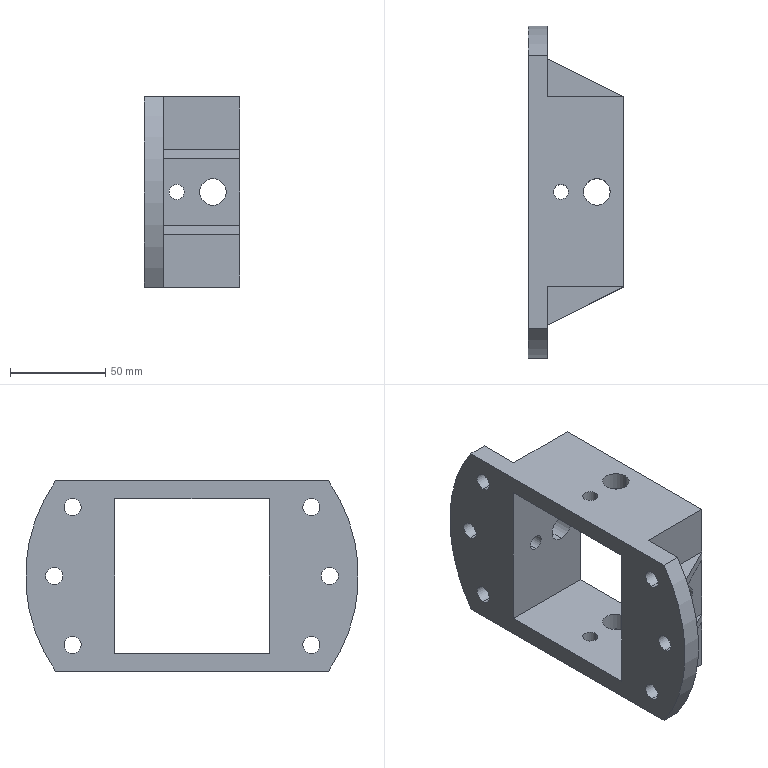Part | SolidWorks | features HoleWzd 4, ICE 4, MirrorPattern 2, Extrusion 1, Rib 1 | 1 solid | 58 faces | box 50 x 175 x 100 mm | volume 233318 mm3 | cylinder 30 | plane 28 | commonest cylinder face diameters 9 x12 8 x8 14 x8 175 x2